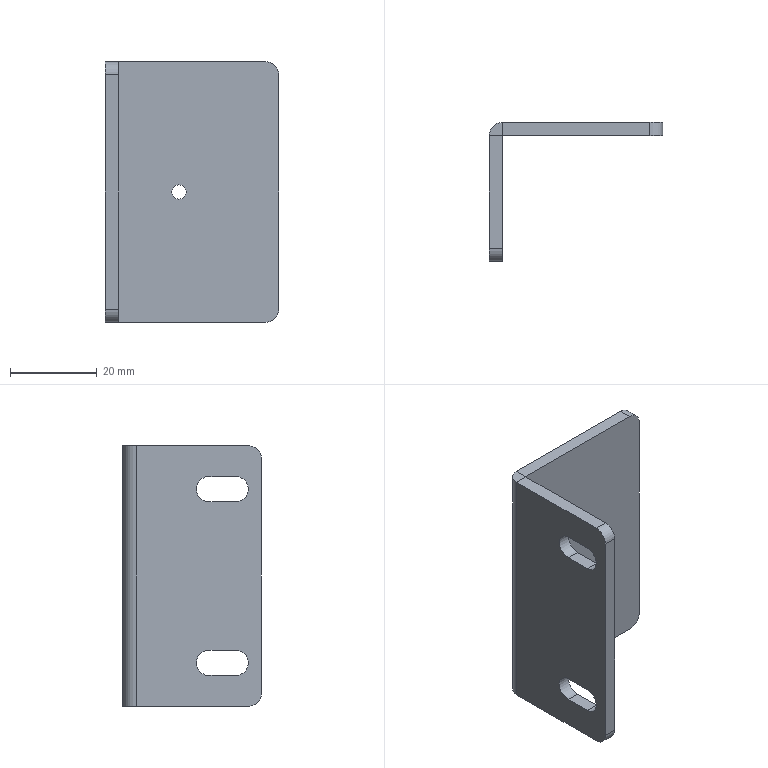Part | STEP file | 1 solid | 28 faces | box 40 x 32 x 60 mm | volume 11873 mm3 | plane 16 | cylinder 12 | commonest cylinder face diameters 5.8 x4 6 x4 3.3 x2 0.2 x1 6.2 x1